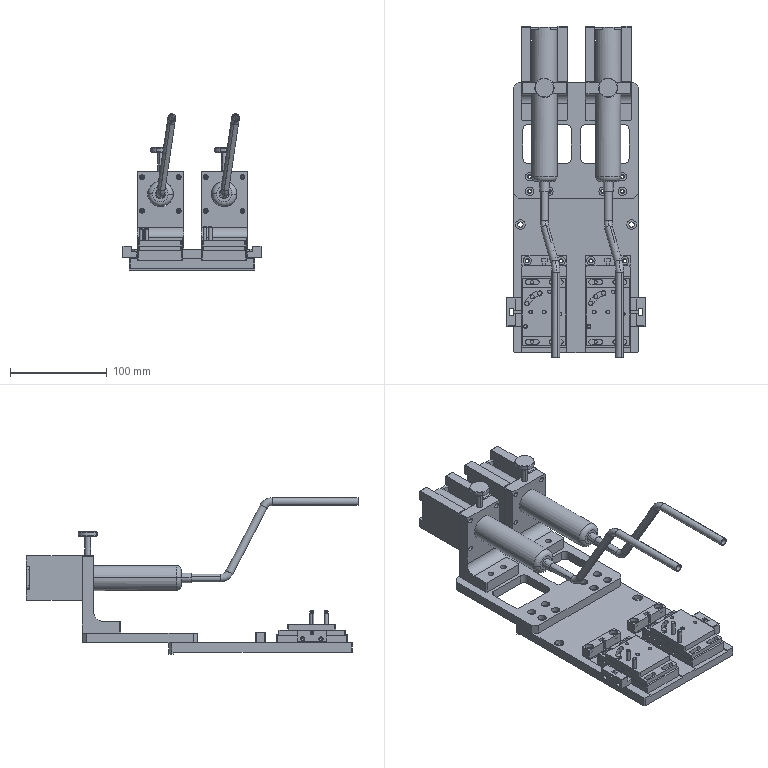Part | NX | features BREP 15 | 31 solids | 904 faces | box 143 x 343.823 x 162.131 mm | volume 751222 mm3 | cylinder 426 | plane 374 | cone 80 | torus 24 | commonest cylinder face diameters 3.3 x88 4.5 x80 6 x40 4 x36 8.6 x24 4.2 x20